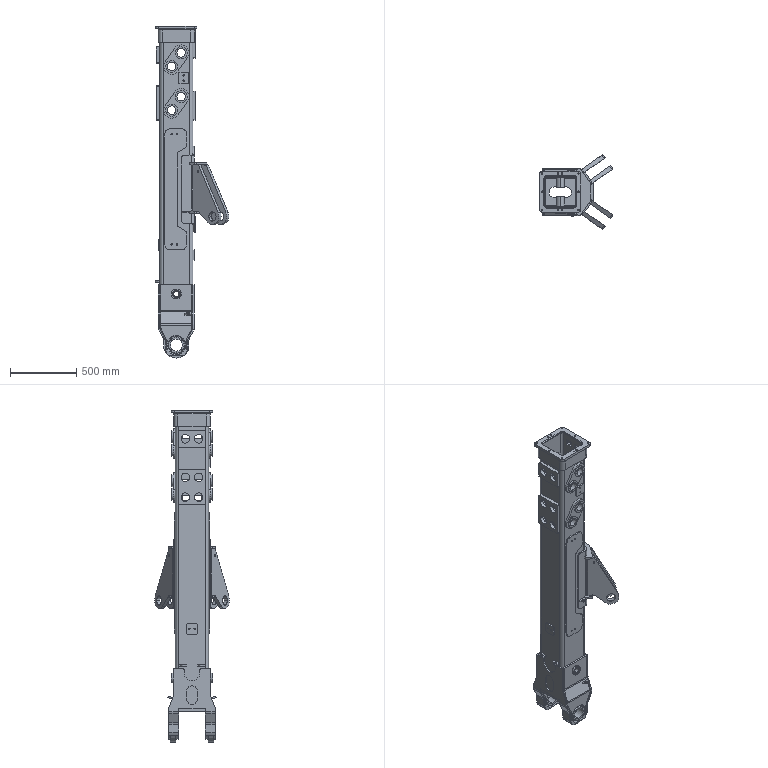Part | SolidWorks | features MirrorCompFeat 3, ReferencePattern 3 | 57 solids | 1360 faces | box 556.673 x 564.682 x 2503 mm | volume 53004232 mm3 | plane 658 | cylinder 516 | cone 178 | spline 8 | commonest cylinder face diameters 10.2 x80 60 x76 80 x72 10 x64 64 x44 20 x20